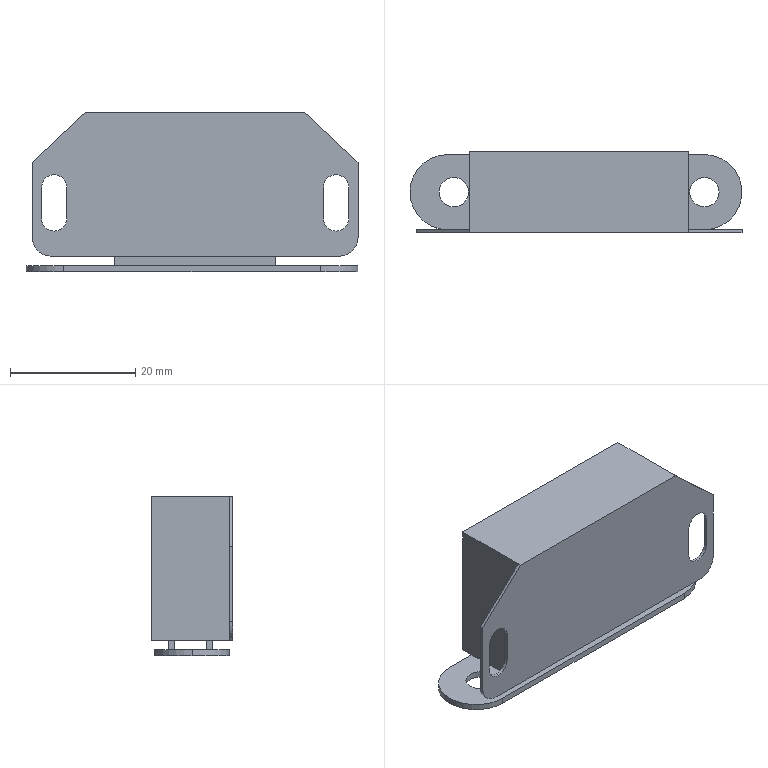Part | STEP file | magnetic door catch | 1 solid | 43 faces | box 53 x 13 x 25.5 mm | volume 11239 mm3 | plane 28 | cylinder 15 | commonest cylinder face diameters 4 x6 4.7 x4 12 x3 6 x2